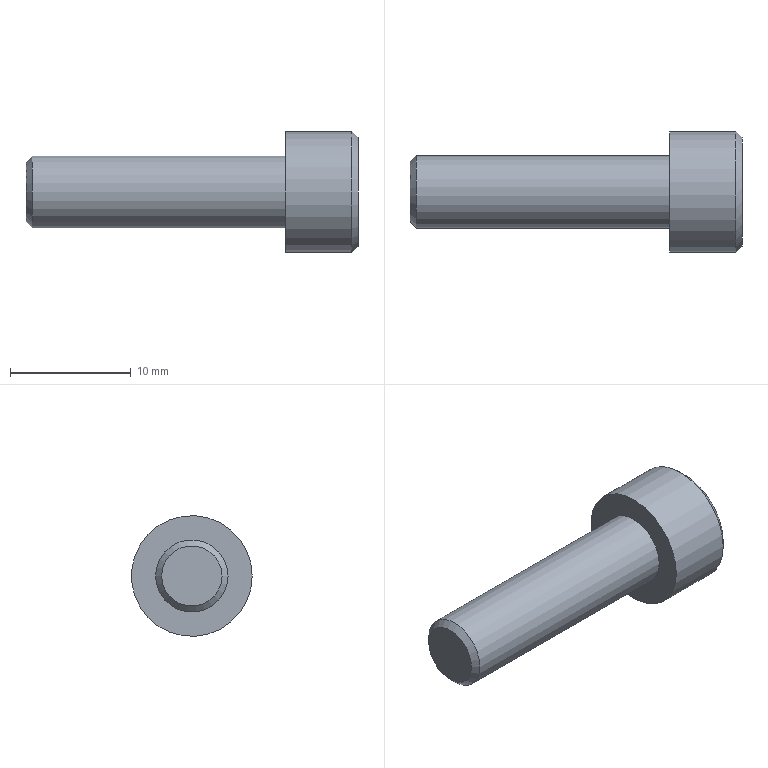Part | STEP file | solid 152 | 1 solid | 14 faces | box 27.5 x 10 x 10 mm | volume 1008 mm3 | plane 10 | cone 2 | cylinder 2 | commonest cylinder face diameters 6 x1 10 x1